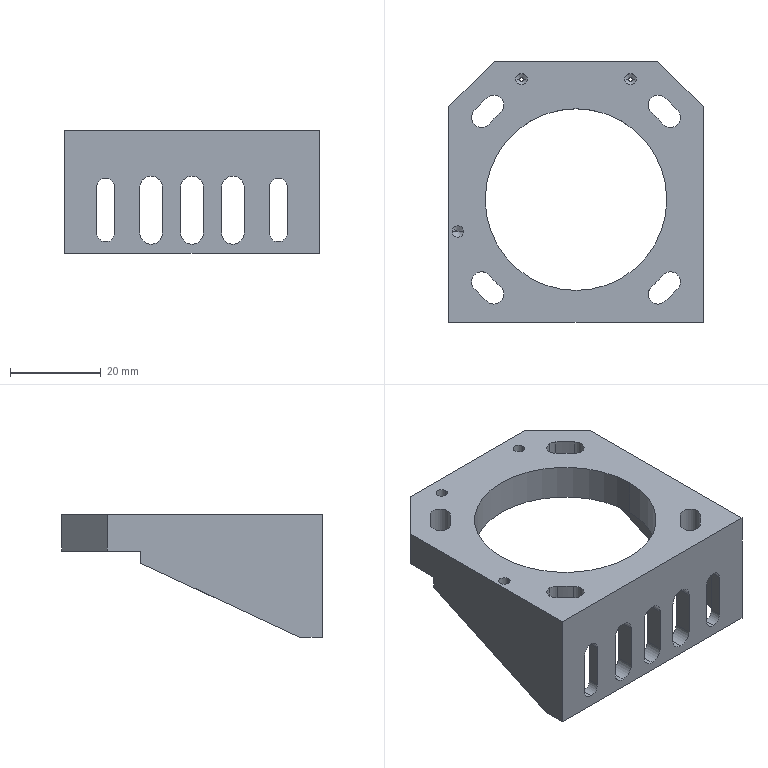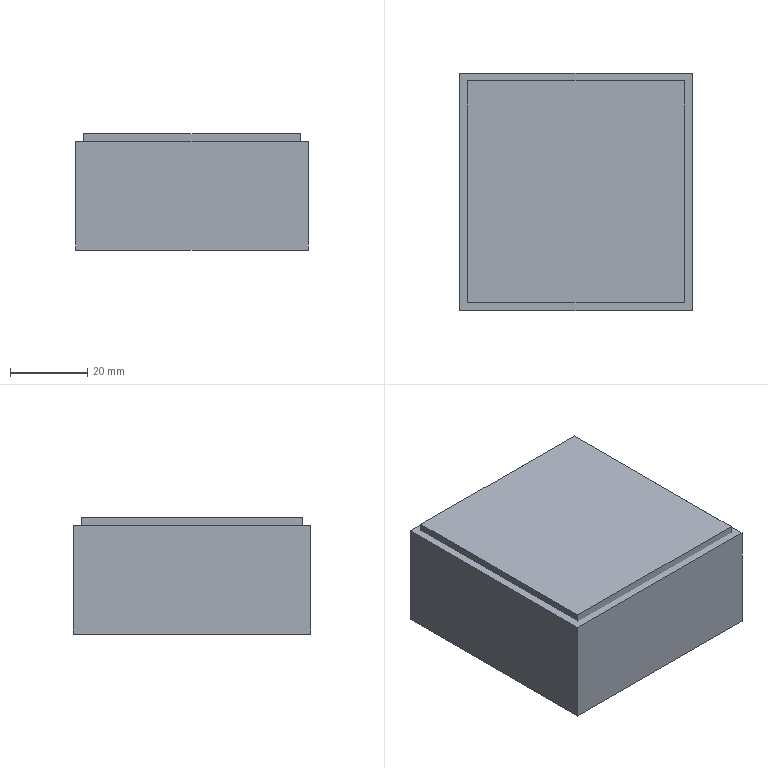CAM job | NX | 3+2 milling, drilling | part box 56 x 57.4 x 27 mm | stock box 60 x 61.4 x 30 mm
Tools:
number,name,description,diameter,corner_radius,flute_length,length,flutes
11,D10JING,Milling Tool-5 Parameters,10.0,0.0,50.0,75.0,2
1,ZXZ,Milling Tool-5 Parameters,6.0,0.0,50.0,75.0,2
12,2.5ZT,Drilling Tool,2.5,0.0,35.0,50.0,2
10,D10C,Milling Tool-5 Parameters,10.0,0.0,50.0,75.0,2
3,D3,Milling Tool-5 Parameters,3.0,0.0,50.0,75.0,2
7,D6A45,Milling Tool-5 Parameters,6.0,0.0,50.0,75.0,2
6,D6JING,Milling Tool-5 Parameters,6.0,0.0,50.0,75.0,2
5,D6R0.5,Milling Tool-5 Parameters,6.0,0.5,50.0,75.0,2
2,D63,Milling Tool-5 Parameters,63.0,0.0,50.0,75.0,2
Operations:
program,operation,operation_type,tool,method,geometry_group,spindle_rpm,surface_speed,feed_per_tooth,feed_cut,feed_plunge,cut_length_mm,path_length_mm,cut_time_min,machine_time_min
1,DRILLING,Operation,ZXZ,METHOD,A,3500.0,65.0,0.0357,250.0,0.0,16.0,181.524,0.064,0.0806
1,DRILLING_COPY,Operation,2.5ZT,METHOD,A,2000.0,15.0,0.03,120.0,0.0,33.753,194.125,0.2813,0.2973
1,ZLEVEL_PROFILE,ZLevelMilling,D10C,METHOD,A,2500.0,78.0,0.5,2500.0,1000.0,66762.735,66846.735,26.723,26.732
1,HOLE_MILLING,CylinderMilling,D10C,METHOD,A,2500.0,78.0,0.44,2200.0,100.0,16196.192,16280.692,7.362,7.37
1,ZLEVEL_PROFILE_COPY,ZLevelMilling,D10JING,METHOD,A,5000.0,157.0,0.12,1200.0,1000.0,764.516,924.235,0.6391,0.6551
1,ZLEVEL_PROFILE_COPY_COPY,ZLevelMilling,D10JING,METHOD,A,5000.0,157.0,0.12,1200.0,1000.0,103.097,176.097,0.0867,0.094
1,ZLEVEL_PROFILE_COPY_1,ZLevelMilling,D3,METHOD,A,5500.0,51.0,0.1136,1250.0,1000.0,8306.85,8693.35,6.659,6.697
1,PLANAR_MILL_COPY,PlanarMilling,D6A45,METHOD,A,7500.0,141.0,0.0833,1250.0,100.0,453.527,1154.098,0.3628,0.4329
2,FLOOR_WALL_COPY,VolumeBased25DMillingOperation,D63,METHOD,B,2000.0,395.0,0.3125,1250.0,100.0,8340.313,10681.637,6.672,6.906
2,FLOOR_WALL_COPY_COPY,VolumeBased25DMillingOperation,D10JING,METHOD,B,5000.0,157.0,0.125,1250.0,100.0,876.797,930.797,0.7014,0.7068
2,FLOOR_WALL_1,VolumeBased25DMillingOperation,D10C,METHOD,B,2500.0,78.0,0.5,2500.0,1000.0,84679.319,89361.718,34.824,35.292
2,CAVITY_MILL,CavityMilling,D10C,METHOD,B,2500.0,78.0,0.44,2200.0,1000.0,17879.575,19757.928,9.377,9.565
2,ZLEVEL_PROFILE_COPY_2,ZLevelMilling,D6JING,METHOD,B,5000.0,94.0,0.15,1500.0,1000.0,4976.215,7585.461,3.731,3.992
2,FLOOR_WALL_2,VolumeBased25DMillingOperation,D6JING,METHOD,B,7000.0,131.0,0.0893,1250.0,100.0,1098.042,1206.877,0.8784,0.8893
2,ZLEVEL_PROFILE_COPY_2_COPY_COPY,ZLevelMilling,D6R0.5,METHOD,B,7000.0,131.0,0.2143,3000.0,1000.0,3212.468,3430.192,1.074,1.096
2,PLANAR_MILL_COPY_COPY,PlanarMilling,D6A45,METHOD,B,7500.0,141.0,0.0833,1250.0,100.0,127.556,253.717,0.102,0.1147
2,PLANAR_MILL_COPY_COPY_COPY,PlanarMilling,D6A45,METHOD,B,7500.0,141.0,0.0833,1250.0,100.0,292.043,975.13,0.2336,0.3019
3,ZLEVEL_PROFILE_COPY_1_COPY,ZLevelMilling,D3,METHOD,C,5500.0,51.0,0.1136,1250.0,1000.0,9984.657,10342.53,8.004,8.04
3,ZLEVEL_PROFILE_COPY_1_COPY_COPY,ZLevelMilling,D3,METHOD,C,7500.0,70.0,0.0667,1000.0,1000.0,89.76,316.511,0.0898,0.1124
3,PLANAR_MILL_COPY_COPY_COPY_1,PlanarMilling,D6A45,METHOD,C,7500.0,141.0,0.0833,1250.0,100.0,180.801,517.043,0.1446,0.1783
3,刀补,ZLevelMilling,D3,METHOD,C,7500.0,70.0,0.0667,1000.0,1000.0,58.683,222.546,0.0587,0.0751